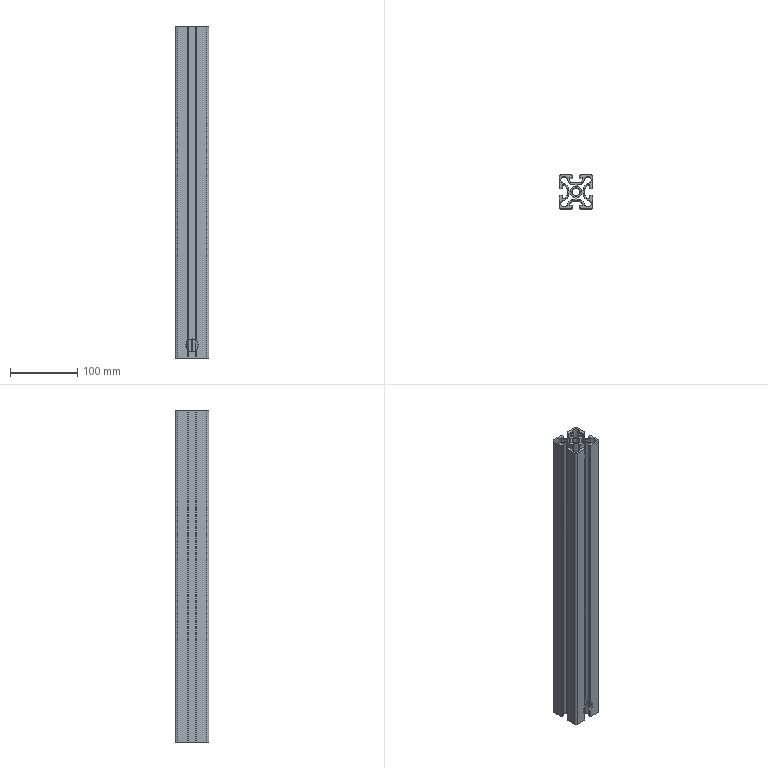Part | NX | features BREP 1 | 1 solid | 189 faces | box 50 x 50 x 495 mm | volume 487265 mm3 | plane 124 | cylinder 65 | commonest cylinder face diameters 2 x33 10 x12 19 x8 6 x4 12 x4 17 x4